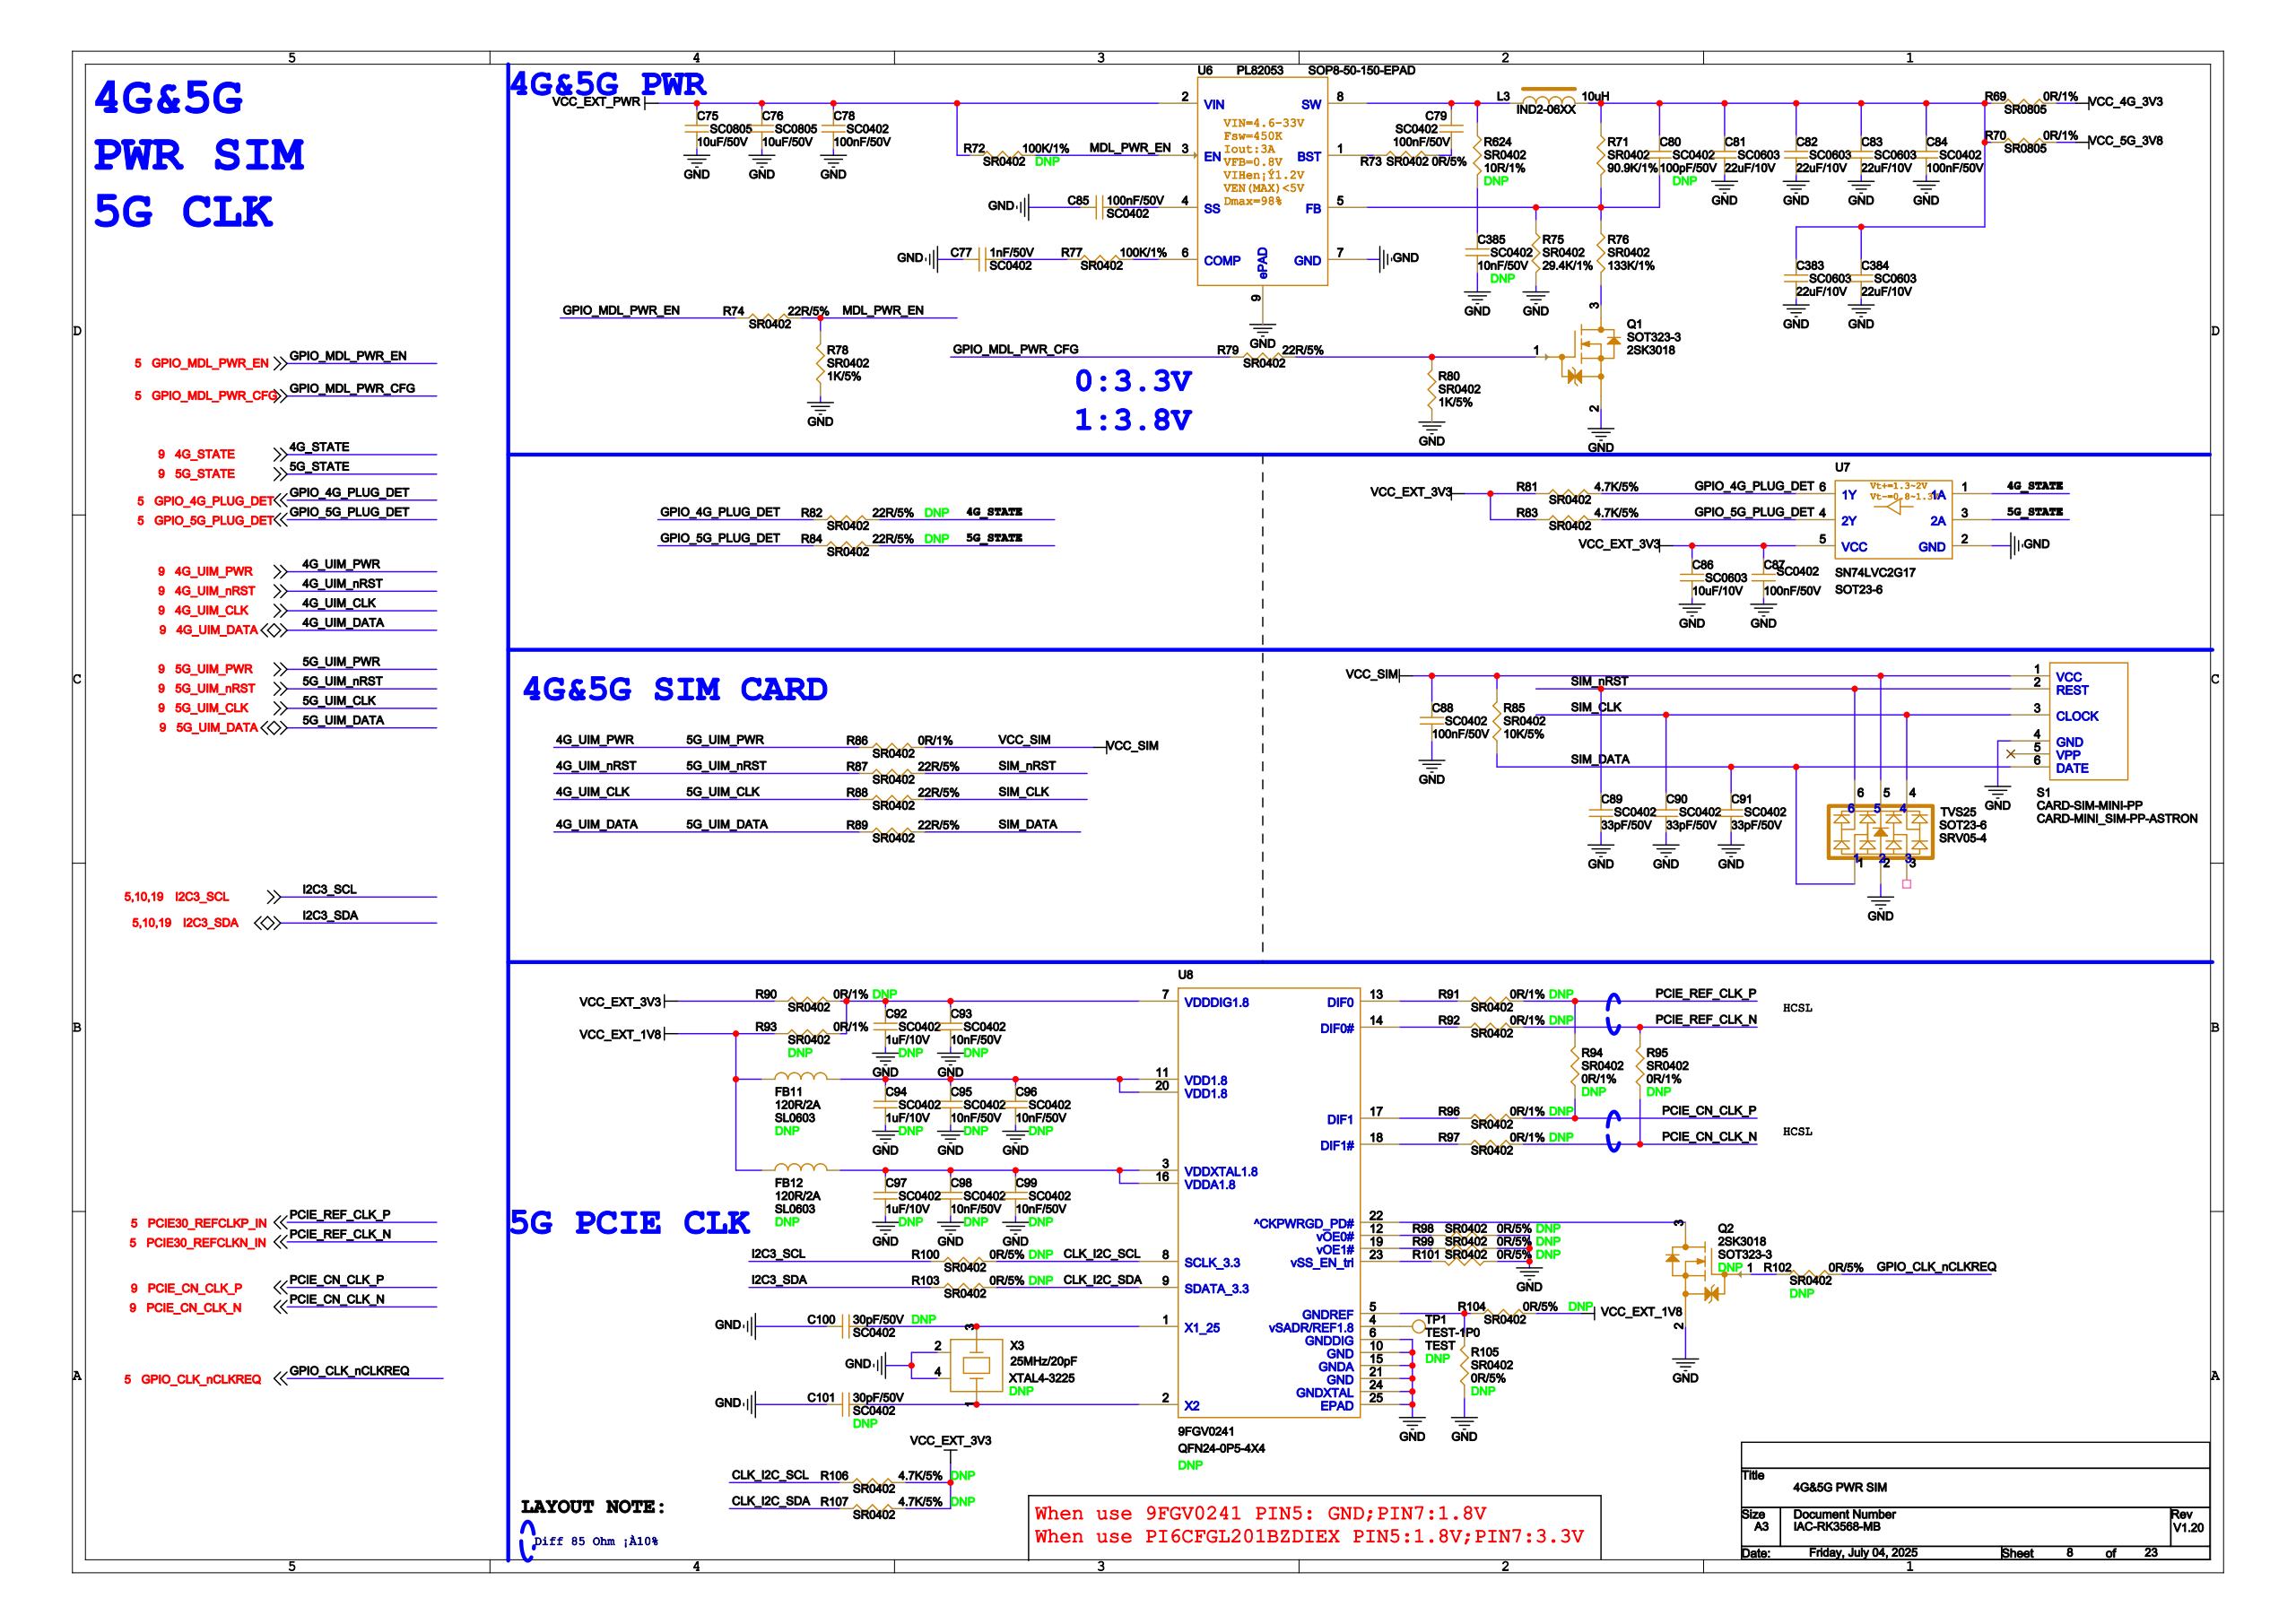Circuit board | Cadence Allegro | 1138 parts | 722 nets | one sheet of the schematic
Parts on this sheet (reference | value | footprint):
C75 | 10uF/50V | SC0805
C76 | 10uF/50V | SC0805
C77 | 1nF/50V | SC0402
C78 | 100nF/50V | SC0402
C80 | 100pF/50V | SC0402
C81 | 22uF/10V | SC0603
C82 | 22uF/10V | SC0603
C83 | 22uF/10V | SC0603
C84 | 100nF/50V | SC0402
C85 | 100nF/50V | SC0402
C86 | 10uF/10V | SC0603
C87 | 100nF/50V | SC0402
C88 | 100nF/50V | SC0402
C89 | 33pF/50V | SC0402
C90 | 33pF/50V | SC0402
C91 | 33pF/50V | SC0402
C92 | 1uF/10V | SC0402
C93 | 10nF/50V | SC0402
C94 | 1uF/10V | SC0402
C95 | 10nF/50V | SC0402
C96 | 10nF/50V | SC0402
C97 | 1uF/10V | SC0402
C98 | 10nF/50V | SC0402
C99 | 10nF/50V | SC0402
C100 | 30pF/50V | SC0402
C101 | 30pF/50V | SC0402
C383 | 22uF/10V | SC0603
C384 | 22uF/10V | SC0603
C385 | 10nF/50V | SC0402
FB11 | 120R/2A | SL0603
FB12 | 120R/2A | SL0603
L3 | 10uH | IND2-06XX
Q1 | 2SK3018 | SOT323-3
Q2 | 2SK3018 | SOT323-3
R69 | 0R/1% | SR0805
R70 | 0R/1% | SR0805
R71 | 90.9K/1% | SR0402
R72 | 100K/1% | SR0402
R73 | 0R/5% | SR0402
R74 | 22R/5% | SR0402
R75 | 29.4K/1% | SR0402
R76 | 133K/1% | SR0402
R77 | 100K/1% | SR0402
R78 | 1K/5% | SR0402
R79 | 22R/5% | SR0402
R80 | 1K/5% | SR0402
R81 | 4.7K/5% | SR0402
R82 | 22R/5% | SR0402
R83 | 4.7K/5% | SR0402
R84 | 22R/5% | SR0402
R85 | 10K/5% | SR0402
R86 | 0R/1% | SR0402
R87 | 22R/5% | SR0402
R88 | 22R/5% | SR0402
R89 | 22R/5% | SR0402
R90 | 0R/1% | SR0402
R91 | 0R/1% | SR0402
R92 | 0R/1% | SR0402
R93 | 0R/1% | SR0402
R94 | 0R/1% | SR0402
R95 | 0R/1% | SR0402
R96 | 0R/1% | SR0402
R97 | 0R/1% | SR0402
R98 | 0R/5% | SR0402
R99 | 0R/5% | SR0402
R100 | 0R/5% | SR0402
R101 | 0R/5% | SR0402
R102 | 0R/5% | SR0402
R103 | 0R/5% | SR0402
R104 | 0R/5% | SR0402
R105 | 0R/5% | SR0402
R106 | 4.7K/5% | SR0402
R107 | 4.7K/5% | SR0402
R624 | 10R/1% | SR0402
S1 | CARD-MINI_SIM-PP-ASTRON | CARD-SIM-MINI-PP
TP1 | TEST | TEST-1P0
TVS25 | SRV05-4 | SOT23-6
U6 | PL82053 | SOP8-50-150-EPAD
U7 | SN74LVC2G17 | SOT23-6
U8 | 9FGV0241 | QFN24-0P5-4X4
X3 | 25MHz/20pF | XTAL4-3225
Nets of these parts (net: part-pin ...):
VCC_EXT_3V3: C86-1 C87-1 R81-1 R83-1 R90-1 R106-2 R107-2 U7-5
GND: C75-2 C76-2 C77-1 C78-2 C81-2 C82-2 C83-2 C84-2 C85-1 C86-2 C87-2 C88-2 C89-1 C90-1 C91-1 C92-2 C93-2 C94-2 C95-2 C96-2 C97-2 C98-2 C99-2 C100-1 C101-1 C383-2 C384-2 C385-2 Q1-2 Q2-2 R75-2 R78-1 R80-1 R98-2 R99-2 R101-2 R105-1 S1-4 TVS25-2 U6-7 U6-9 U7-2 X3-2 X3-4 U8-6 U8-10 U8-15 U8-21 U8-24 U8-25
SIM_DATA: C91-2 R85-1 R89-2 S1-6 TVS25-1
SIM_CLK: C90-2 R88-2 S1-3 TVS25-4
VCC_SIM: C88-1 R85-2 R86-2 S1-1 TVS25-5
SIM_NRST: C89-2 R87-2 S1-2 TVS25-6
VCC_EXT_PWR: C75-1 C76-1 C78-1 R72-1 U6-2
N3996667: L3-1 R624-1 U6-8
N7444516: C385-1 R624-2
N3996663: C80-1 C81-1 C82-1 C83-1 C84-1 C383-1 C384-1 L3-2 R69-1 R70-1 R71-1
N3996739: C80-2 R71-2 R75-1 R76-1 U6-5
N4012620: Q1-3 R76-2
N3996731: R73-1 U6-1
MDL_PWR_EN: R72-2 R74-2 R78-2 U6-3
N4000351: C85-2 U6-4
N3996755: R77-2 U6-6
4G_STATE: R82-2 U7-1
VCC_4G_3V3: R69-2
4G_UIM_CLK: R88-1
4G_UIM_DATA: R89-1
4G_UIM_NRST: R87-1
4G_UIM_PWR: R86-1
VCC_5G_3V8: R70-2
5G_STATE: R84-2 U7-3
VCC_EXT_1V8: FB11-1 FB12-1 R93-1 R104-2
N4012705: Q1-1 R79-2 R80-2
N4014162: Q2-3 U8-22
N4014198: Q2-1 R102-1
N4014228: C100-2 X3-3 U8-1
N4014232: C101-2 X3-1 U8-2
N4014128: C92-1 C93-1 R90-2 R93-2 U8-7
N4014666: C94-1 C95-1 C96-1 FB11-2 U8-11 U8-20
N4014812: C97-1 C98-1 C99-1 FB12-2 U8-3 U8-16
N7439737: C77-2 R77-1
N4015172: R91-1 U8-13
PCIE30_REFCLKP_IN: R91-2 R94-2
N4015168: R92-1 U8-14
PCIE30_REFCLKN_IN: R92-2 R95-2
PCIE_CN_CLK_P: R94-1 R96-2
PCIE_CN_CLK_N: R95-1 R97-2
N4015136: R96-1 U8-17
N4015132: R97-1 U8-18
N401455616: TP1-1 U8-4
GPIO_5G_PLUG_DET: R83-2 R84-1 U7-4
GPIO_CLK_NCLKREQ: R102-2
GPIO_MDL_PWR_CFG: R79-1
I2C3_SCL: R100-1
I2C3_SDA: R103-1
GPIO_MDL_PWR_EN: R74-1
GPIO_4G_PLUG_DET: R81-2 R82-1 U7-6
N4014412: R104-1 R105-2 U8-5
CLK_I2C_SCL: R100-2 R106-1 U8-8
CLK_I2C_SDA: R103-2 R107-1 U8-9
N4014994: R98-1 U8-12
N4015046: R99-1 U8-19
N4015090: R101-1 U8-23
N3996649: R73-2